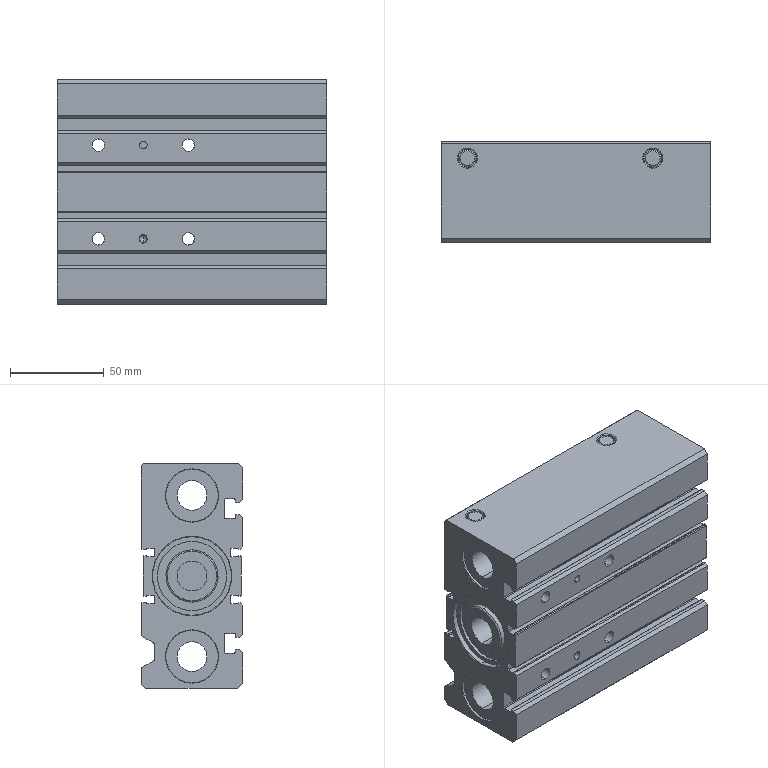Part | NX | features BREP 1 | 1 solid | 292 faces | box 144 x 54 x 120 mm | volume 611114 mm3 | cylinder 132 | plane 96 | cone 60 | torus 4 | commonest cylinder face diameters 0.8 x28 6.647 x16 4 x14 0.4 x12 6.5 x8 11 x8